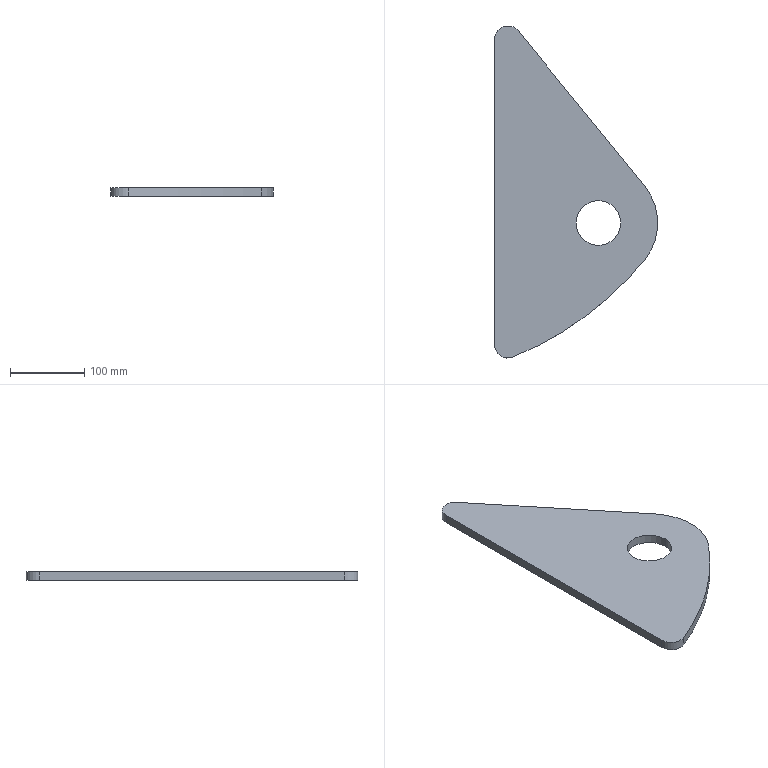Part | SolidWorks | features Extrusion 1 | 1 solid | 10 faces | box 220 x 447.752 x 12 mm | volume 720833 mm3 | cylinder 6 | plane 4 | commonest cylinder face diameters 36 x2 60 x2 160 x1 900 x1
STEP:
#1=CARTESIAN_POINT('',(-30.,0.,12.));
#2=VERTEX_POINT('',#1);
#3=CARTESIAN_POINT('',(30.,0.,12.));
#4=VERTEX_POINT('',#3);
#5=CARTESIAN_POINT('',(0.,0.,12.));
#6=DIRECTION('',(0.,0.,1.));
#7=DIRECTION('',(1.,0.,0.));
#8=AXIS2_PLACEMENT_3D('',#5,#6,#7);
#9=CIRCLE('',#8,30.);
#10=EDGE_CURVE('',#2,#4,#9,.T.);
#11=ORIENTED_EDGE('',*,*,#10,.T.);
#12=CARTESIAN_POINT('',(30.,0.,0.));
#13=VERTEX_POINT('',#12);
#14=CARTESIAN_POINT('',(30.,0.,12.));
#15=DIRECTION('',(0.,0.,-1.));
#16=VECTOR('',#15,1000.);
#17=LINE('',#14,#16);
#18=EDGE_CURVE('',#4,#13,#17,.T.);
#19=ORIENTED_EDGE('',*,*,#18,.T.);
#20=CARTESIAN_POINT('',(-30.,0.,0.));
#21=VERTEX_POINT('',#20);
#22=CARTESIAN_POINT('',(0.,0.,0.));
#23=DIRECTION('',(0.,0.,1.));
#24=DIRECTION('',(1.,0.,0.));
#25=AXIS2_PLACEMENT_3D('',#22,#23,#24);
#26=CIRCLE('',#25,30.);
#27=EDGE_CURVE('',#21,#13,#26,.T.);
#28=ORIENTED_EDGE('',*,*,#27,.F.);
#29=CARTESIAN_POINT('',(-30.,0.,12.));
#30=DIRECTION('',(0.,0.,-1.));
#31=VECTOR('',#30,1000.);
#32=LINE('',#29,#31);
#33=EDGE_CURVE('',#2,#21,#32,.T.);
#34=ORIENTED_EDGE('',*,*,#33,.F.);
#35=EDGE_LOOP('',(#11,#19,#28,#34));
#36=FACE_OUTER_BOUND('',#35,.T.);
#37=CARTESIAN_POINT('',(0.,0.,12.));
#38=DIRECTION('',(0.,0.,-1.));
#39=DIRECTION('',(-1.,0.,0.));
#40=AXIS2_PLACEMENT_3D('',#37,#38,#39);
#41=CYLINDRICAL_SURFACE('',#40,30.);
#42=ADVANCED_FACE('',(#36),#41,.F.);
#43=CARTESIAN_POINT('',(-140.,-164.069,12.));
#44=VERTEX_POINT('',#43);
#45=CARTESIAN_POINT('',(-115.208,-180.738,12.));
#46=VERTEX_POINT('',#45);
#47=CARTESIAN_POINT('',(-122.,-164.069,12.));
#48=DIRECTION('',(0.,0.,1.));
#49=DIRECTION('',(1.,0.,0.));
#50=AXIS2_PLACEMENT_3D('',#47,#48,#49);
#51=CIRCLE('',#50,18.);
#52=EDGE_CURVE('',#44,#46,#51,.T.);
#53=ORIENTED_EDGE('',*,*,#52,.T.);
#54=CARTESIAN_POINT('',(63.089,-49.191,12.));
#55=VERTEX_POINT('',#54);
#56=CARTESIAN_POINT('',(-285.,236.,12.));
#57=DIRECTION('',(0.,0.,1.));
#58=DIRECTION('',(1.,0.,0.));
#59=AXIS2_PLACEMENT_3D('',#56,#57,#58);
#60=CIRCLE('',#59,450.);
#61=EDGE_CURVE('',#46,#55,#60,.T.);
#62=ORIENTED_EDGE('',*,*,#61,.T.);
#63=CARTESIAN_POINT('',(61.996,50.562,12.));
#64=VERTEX_POINT('',#63);
#65=CARTESIAN_POINT('',(0.,0.,12.));
#66=DIRECTION('',(0.,0.,1.));
#67=DIRECTION('',(1.,0.,0.));
#68=AXIS2_PLACEMENT_3D('',#65,#66,#67);
#69=CIRCLE('',#68,80.);
#70=EDGE_CURVE('',#55,#64,#69,.T.);
#71=ORIENTED_EDGE('',*,*,#70,.T.);
#72=CARTESIAN_POINT('',(-108.051,259.06,12.));
#73=VERTEX_POINT('',#72);
#74=CARTESIAN_POINT('',(61.996,50.562,12.));
#75=DIRECTION('',(-0.632,0.7749,0.));
#76=VECTOR('',#75,1000.);
#77=LINE('',#74,#76);
#78=EDGE_CURVE('',#64,#73,#77,.T.);
#79=ORIENTED_EDGE('',*,*,#78,.T.);
#80=CARTESIAN_POINT('',(-140.,247.683,12.));
#81=VERTEX_POINT('',#80);
#82=CARTESIAN_POINT('',(-122.,247.683,12.));
#83=DIRECTION('',(0.,0.,1.));
#84=DIRECTION('',(-1.,0.,0.));
#85=AXIS2_PLACEMENT_3D('',#82,#83,#84);
#86=CIRCLE('',#85,18.);
#87=EDGE_CURVE('',#73,#81,#86,.T.);
#88=ORIENTED_EDGE('',*,*,#87,.T.);
#89=CARTESIAN_POINT('',(-140.,247.683,12.));
#90=DIRECTION('',(0.,-1.,0.));
#91=VECTOR('',#90,1000.);
#92=LINE('',#89,#91);
#93=EDGE_CURVE('',#81,#44,#92,.T.);
#94=ORIENTED_EDGE('',*,*,#93,.T.);
#95=EDGE_LOOP('',(#53,#62,#71,#79,#88,#94));
#96=FACE_OUTER_BOUND('',#95,.T.);
#97=ORIENTED_EDGE('',*,*,#10,.F.);
#98=CARTESIAN_POINT('',(0.,0.,12.));
#99=DIRECTION('',(0.,0.,1.));
#100=DIRECTION('',(1.,0.,0.));
#101=AXIS2_PLACEMENT_3D('',#98,#99,#100);
#102=CIRCLE('',#101,30.);
#103=EDGE_CURVE('',#4,#2,#102,.T.);
#104=ORIENTED_EDGE('',*,*,#103,.F.);
#105=EDGE_LOOP('',(#97,#104));
#106=FACE_BOUND('',#105,.T.);
#107=CARTESIAN_POINT('',(-122.,-164.069,12.));
#108=DIRECTION('',(0.,0.,1.));
#109=DIRECTION('',(1.,0.,0.));
#110=AXIS2_PLACEMENT_3D('',#107,#108,#109);
#111=PLANE('',#110);
#112=ADVANCED_FACE('',(#96,#106),#111,.T.);
#113=CARTESIAN_POINT('',(-140.,-164.069,0.));
#114=VERTEX_POINT('',#113);
#115=CARTESIAN_POINT('',(-115.208,-180.738,0.));
#116=VERTEX_POINT('',#115);
#117=CARTESIAN_POINT('',(-122.,-164.069,0.));
#118=DIRECTION('',(0.,0.,1.));
#119=DIRECTION('',(1.,0.,0.));
#120=AXIS2_PLACEMENT_3D('',#117,#118,#119);
#121=CIRCLE('',#120,18.);
#122=EDGE_CURVE('',#114,#116,#121,.T.);
#123=ORIENTED_EDGE('',*,*,#122,.F.);
#124=CARTESIAN_POINT('',(-140.,247.683,0.));
#125=VERTEX_POINT('',#124);
#126=CARTESIAN_POINT('',(-140.,247.683,0.));
#127=DIRECTION('',(0.,-1.,0.));
#128=VECTOR('',#127,1000.);
#129=LINE('',#126,#128);
#130=EDGE_CURVE('',#125,#114,#129,.T.);
#131=ORIENTED_EDGE('',*,*,#130,.F.);
#132=CARTESIAN_POINT('',(-108.051,259.06,0.));
#133=VERTEX_POINT('',#132);
#134=CARTESIAN_POINT('',(-122.,247.683,0.));
#135=DIRECTION('',(0.,0.,1.));
#136=DIRECTION('',(-1.,0.,0.));
#137=AXIS2_PLACEMENT_3D('',#134,#135,#136);
#138=CIRCLE('',#137,18.);
#139=EDGE_CURVE('',#133,#125,#138,.T.);
#140=ORIENTED_EDGE('',*,*,#139,.F.);
#141=CARTESIAN_POINT('',(61.996,50.562,0.));
#142=VERTEX_POINT('',#141);
#143=CARTESIAN_POINT('',(61.996,50.562,0.));
#144=DIRECTION('',(-0.632,0.7749,0.));
#145=VECTOR('',#144,1000.);
#146=LINE('',#143,#145);
#147=EDGE_CURVE('',#142,#133,#146,.T.);
#148=ORIENTED_EDGE('',*,*,#147,.F.);
#149=CARTESIAN_POINT('',(63.089,-49.191,0.));
#150=VERTEX_POINT('',#149);
#151=CARTESIAN_POINT('',(0.,0.,0.));
#152=DIRECTION('',(0.,0.,1.));
#153=DIRECTION('',(1.,0.,0.));
#154=AXIS2_PLACEMENT_3D('',#151,#152,#153);
#155=CIRCLE('',#154,80.);
#156=EDGE_CURVE('',#150,#142,#155,.T.);
#157=ORIENTED_EDGE('',*,*,#156,.F.);
#158=CARTESIAN_POINT('',(-285.,236.,0.));
#159=DIRECTION('',(0.,0.,1.));
#160=DIRECTION('',(1.,0.,0.));
#161=AXIS2_PLACEMENT_3D('',#158,#159,#160);
#162=CIRCLE('',#161,450.);
#163=EDGE_CURVE('',#116,#150,#162,.T.);
#164=ORIENTED_EDGE('',*,*,#163,.F.);
#165=EDGE_LOOP('',(#123,#131,#140,#148,#157,#164));
#166=FACE_OUTER_BOUND('',#165,.T.);
#167=ORIENTED_EDGE('',*,*,#27,.T.);
#168=CARTESIAN_POINT('',(0.,0.,0.));
#169=DIRECTION('',(0.,0.,1.));
#170=DIRECTION('',(1.,0.,0.));
#171=AXIS2_PLACEMENT_3D('',#168,#169,#170);
#172=CIRCLE('',#171,30.);
#173=EDGE_CURVE('',#13,#21,#172,.T.);
#174=ORIENTED_EDGE('',*,*,#173,.T.);
#175=EDGE_LOOP('',(#167,#174));
#176=FACE_BOUND('',#175,.T.);
#177=CARTESIAN_POINT('',(-122.,-164.069,0.));
#178=DIRECTION('',(0.,0.,1.));
#179=DIRECTION('',(1.,0.,0.));
#180=AXIS2_PLACEMENT_3D('',#177,#178,#179);
#181=PLANE('',#180);
#182=ADVANCED_FACE('',(#166,#176),#181,.F.);
#183=ORIENTED_EDGE('',*,*,#122,.T.);
#184=CARTESIAN_POINT('',(-115.208,-180.738,12.));
#185=DIRECTION('',(0.,0.,-1.));
#186=VECTOR('',#185,1000.);
#187=LINE('',#184,#186);
#188=EDGE_CURVE('',#46,#116,#187,.T.);
#189=ORIENTED_EDGE('',*,*,#188,.F.);
#190=ORIENTED_EDGE('',*,*,#52,.F.);
#191=CARTESIAN_POINT('',(-140.,-164.069,12.));
#192=DIRECTION('',(0.,0.,-1.));
#193=VECTOR('',#192,1000.);
#194=LINE('',#191,#193);
#195=EDGE_CURVE('',#44,#114,#194,.T.);
#196=ORIENTED_EDGE('',*,*,#195,.T.);
#197=EDGE_LOOP('',(#183,#189,#190,#196));
#198=FACE_OUTER_BOUND('',#197,.T.);
#199=CARTESIAN_POINT('',(-122.,-164.069,12.));
#200=DIRECTION('',(0.,0.,-1.));
#201=DIRECTION('',(-1.,0.,0.));
#202=AXIS2_PLACEMENT_3D('',#199,#200,#201);
#203=CYLINDRICAL_SURFACE('',#202,18.);
#204=ADVANCED_FACE('',(#198),#203,.T.);
#205=ORIENTED_EDGE('',*,*,#163,.T.);
#206=CARTESIAN_POINT('',(63.089,-49.191,12.));
#207=DIRECTION('',(0.,0.,-1.));
#208=VECTOR('',#207,1000.);
#209=LINE('',#206,#208);
#210=EDGE_CURVE('',#55,#150,#209,.T.);
#211=ORIENTED_EDGE('',*,*,#210,.F.);
#212=ORIENTED_EDGE('',*,*,#61,.F.);
#213=ORIENTED_EDGE('',*,*,#188,.T.);
#214=EDGE_LOOP('',(#205,#211,#212,#213));
#215=FACE_OUTER_BOUND('',#214,.T.);
#216=CARTESIAN_POINT('',(-285.,236.,12.));
#217=DIRECTION('',(0.,0.,-1.));
#218=DIRECTION('',(-1.,0.,0.));
#219=AXIS2_PLACEMENT_3D('',#216,#217,#218);
#220=CYLINDRICAL_SURFACE('',#219,450.);
#221=ADVANCED_FACE('',(#215),#220,.T.);
#222=ORIENTED_EDGE('',*,*,#156,.T.);
#223=CARTESIAN_POINT('',(61.996,50.562,12.));
#224=DIRECTION('',(0.,0.,-1.));
#225=VECTOR('',#224,1000.);
#226=LINE('',#223,#225);
#227=EDGE_CURVE('',#64,#142,#226,.T.);
#228=ORIENTED_EDGE('',*,*,#227,.F.);
#229=ORIENTED_EDGE('',*,*,#70,.F.);
#230=ORIENTED_EDGE('',*,*,#210,.T.);
#231=EDGE_LOOP('',(#222,#228,#229,#230));
#232=FACE_OUTER_BOUND('',#231,.T.);
#233=CARTESIAN_POINT('',(0.,0.,12.));
#234=DIRECTION('',(0.,0.,-1.));
#235=DIRECTION('',(-1.,0.,0.));
#236=AXIS2_PLACEMENT_3D('',#233,#234,#235);
#237=CYLINDRICAL_SURFACE('',#236,80.);
#238=ADVANCED_FACE('',(#232),#237,.T.);
#239=ORIENTED_EDGE('',*,*,#147,.T.);
#240=CARTESIAN_POINT('',(-108.051,259.06,12.));
#241=DIRECTION('',(0.,0.,-1.));
#242=VECTOR('',#241,1000.);
#243=LINE('',#240,#242);
#244=EDGE_CURVE('',#73,#133,#243,.T.);
#245=ORIENTED_EDGE('',*,*,#244,.F.);
#246=ORIENTED_EDGE('',*,*,#78,.F.);
#247=ORIENTED_EDGE('',*,*,#227,.T.);
#248=EDGE_LOOP('',(#239,#245,#246,#247));
#249=FACE_OUTER_BOUND('',#248,.T.);
#250=CARTESIAN_POINT('',(61.996,50.562,12.));
#251=DIRECTION('',(-0.7749,-0.632,0.));
#252=DIRECTION('',(0.632,-0.7749,0.));
#253=AXIS2_PLACEMENT_3D('',#250,#251,#252);
#254=PLANE('',#253);
#255=ADVANCED_FACE('',(#249),#254,.F.);
#256=ORIENTED_EDGE('',*,*,#139,.T.);
#257=CARTESIAN_POINT('',(-140.,247.683,12.));
#258=DIRECTION('',(0.,0.,-1.));
#259=VECTOR('',#258,1000.);
#260=LINE('',#257,#259);
#261=EDGE_CURVE('',#81,#125,#260,.T.);
#262=ORIENTED_EDGE('',*,*,#261,.F.);
#263=ORIENTED_EDGE('',*,*,#87,.F.);
#264=ORIENTED_EDGE('',*,*,#244,.T.);
#265=EDGE_LOOP('',(#256,#262,#263,#264));
#266=FACE_OUTER_BOUND('',#265,.T.);
#267=CARTESIAN_POINT('',(-122.,247.683,12.));
#268=DIRECTION('',(0.,0.,-1.));
#269=DIRECTION('',(-1.,0.,0.));
#270=AXIS2_PLACEMENT_3D('',#267,#268,#269);
#271=CYLINDRICAL_SURFACE('',#270,18.);
#272=ADVANCED_FACE('',(#266),#271,.T.);
#273=ORIENTED_EDGE('',*,*,#130,.T.);
#274=ORIENTED_EDGE('',*,*,#195,.F.);
#275=ORIENTED_EDGE('',*,*,#93,.F.);
#276=ORIENTED_EDGE('',*,*,#261,.T.);
#277=EDGE_LOOP('',(#273,#274,#275,#276));
#278=FACE_OUTER_BOUND('',#277,.T.);
#279=CARTESIAN_POINT('',(-140.,247.683,12.));
#280=DIRECTION('',(1.,0.,0.));
#281=DIRECTION('',(0.,1.,0.));
#282=AXIS2_PLACEMENT_3D('',#279,#280,#281);
#283=PLANE('',#282);
#284=ADVANCED_FACE('',(#278),#283,.F.);
#285=ORIENTED_EDGE('',*,*,#18,.F.);
#286=ORIENTED_EDGE('',*,*,#103,.T.);
#287=ORIENTED_EDGE('',*,*,#33,.T.);
#288=ORIENTED_EDGE('',*,*,#173,.F.);
#289=EDGE_LOOP('',(#285,#286,#287,#288));
#290=FACE_OUTER_BOUND('',#289,.T.);
#291=CARTESIAN_POINT('',(0.,0.,12.));
#292=DIRECTION('',(0.,0.,-1.));
#293=DIRECTION('',(-1.,0.,0.));
#294=AXIS2_PLACEMENT_3D('',#291,#292,#293);
#295=CYLINDRICAL_SURFACE('',#294,30.);
#296=ADVANCED_FACE('',(#290),#295,.F.);
#297=CLOSED_SHELL('',(#42,#112,#182,#204,#221,#238,#255,#272,#284,#296));
#298=MANIFOLD_SOLID_BREP('',#297);
#299=CARTESIAN_POINT('',(0.,0.,0.));
#300=DIRECTION('',(0.,0.,1.));
#301=DIRECTION('',(1.,0.,0.));
#302=AXIS2_PLACEMENT_3D('',#299,#300,#301);
#303=(LENGTH_UNIT()NAMED_UNIT(*)SI_UNIT(.MILLI.,.METRE.));
#304=UNCERTAINTY_MEASURE_WITH_UNIT(LENGTH_MEASURE(0.00001),#303,'','');
#305=(NAMED_UNIT(*)PLANE_ANGLE_UNIT()SI_UNIT($,.RADIAN.));
#306=(NAMED_UNIT(*)SI_UNIT($,.STERADIAN.)SOLID_ANGLE_UNIT());
#307=(GEOMETRIC_REPRESENTATION_CONTEXT(3)GLOBAL_UNCERTAINTY_ASSIGNED_CONTEXT((#304))GLOBAL_UNIT_ASSIGNED_CONTEXT((#303,#305,#306))REPRESENTATION_CONTEXT('',''));
#308=ADVANCED_BREP_SHAPE_REPRESENTATION('',(#298,#302),#307);